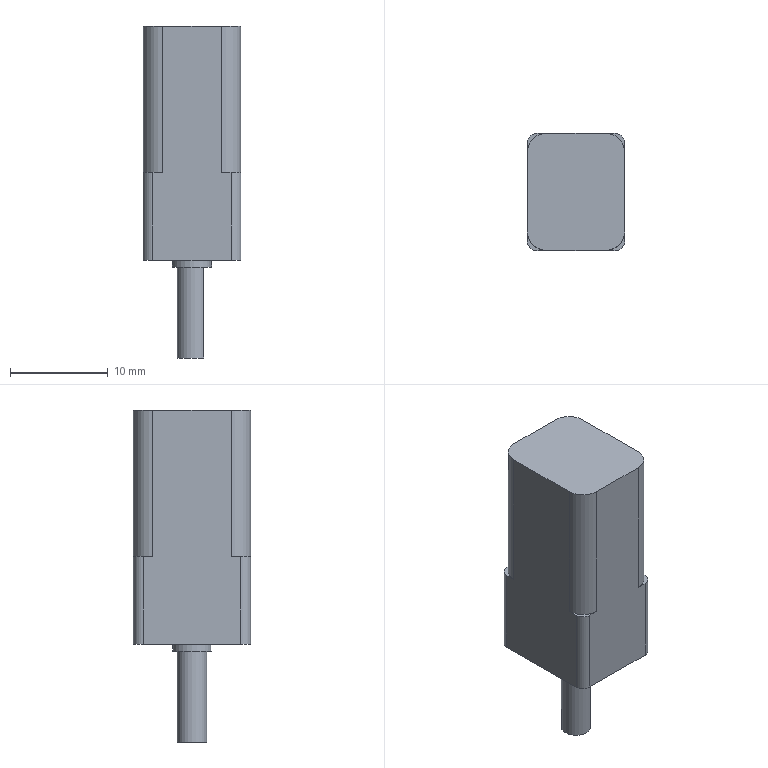Part | NX | features DATUM_CSYS 4, EXTRUDE 4, SKETCH 3, BLEND 2, UNITE 2 | 2 solids | 24 faces | box 10 x 12 x 34 mm | volume 2897 mm3 | plane 14 | cylinder 10 | commonest cylinder face diameters 4 x5 2 x4 3 x1
STEP:
#1=CARTESIAN_POINT('',(1.2,-0.9,-9.));
#2=VERTEX_POINT('',#1);
#3=CARTESIAN_POINT('',(1.2,0.9,-9.));
#4=VERTEX_POINT('',#3);
#5=CARTESIAN_POINT('',(0.,0.,-9.));
#6=DIRECTION('',(0.,0.,-1.));
#7=DIRECTION('',(1.,0.,0.));
#8=AXIS2_PLACEMENT_3D('',#5,#6,#7);
#9=CIRCLE('',#8,1.5);
#10=EDGE_CURVE('',#2,#4,#9,.T.);
#11=ORIENTED_EDGE('',*,*,#10,.T.);
#12=CARTESIAN_POINT('',(1.2,0.9,-19.));
#13=VERTEX_POINT('',#12);
#14=CARTESIAN_POINT('',(1.2,0.9,-19.));
#15=DIRECTION('',(0.,0.,1.));
#16=VECTOR('',#15,1000.);
#17=LINE('',#14,#16);
#18=EDGE_CURVE('',#13,#4,#17,.T.);
#19=ORIENTED_EDGE('',*,*,#18,.F.);
#20=CARTESIAN_POINT('',(1.2,-0.9,-19.));
#21=VERTEX_POINT('',#20);
#22=CARTESIAN_POINT('',(0.,0.,-19.));
#23=DIRECTION('',(0.,0.,-1.));
#24=DIRECTION('',(1.,0.,0.));
#25=AXIS2_PLACEMENT_3D('',#22,#23,#24);
#26=CIRCLE('',#25,1.5);
#27=EDGE_CURVE('',#21,#13,#26,.T.);
#28=ORIENTED_EDGE('',*,*,#27,.F.);
#29=CARTESIAN_POINT('',(1.2,-0.9,-19.));
#30=DIRECTION('',(0.,0.,1.));
#31=VECTOR('',#30,1000.);
#32=LINE('',#29,#31);
#33=EDGE_CURVE('',#2,#21,#32,.F.);
#34=ORIENTED_EDGE('',*,*,#33,.F.);
#35=EDGE_LOOP('',(#11,#19,#28,#34));
#36=FACE_BOUND('',#35,.T.);
#37=CARTESIAN_POINT('',(0.,0.,-19.));
#38=DIRECTION('',(0.,0.,1.));
#39=DIRECTION('',(1.,0.,0.));
#40=AXIS2_PLACEMENT_3D('',#37,#38,#39);
#41=CYLINDRICAL_SURFACE('',#40,1.5);
#42=ADVANCED_FACE('',(#36),#41,.T.);
#43=CARTESIAN_POINT('',(1.2,0.9,-9.));
#44=DIRECTION('',(0.,-1.,0.));
#45=VECTOR('',#44,1000.);
#46=LINE('',#43,#45);
#47=EDGE_CURVE('',#4,#2,#46,.T.);
#48=ORIENTED_EDGE('',*,*,#47,.T.);
#49=ORIENTED_EDGE('',*,*,#33,.T.);
#50=CARTESIAN_POINT('',(1.2,0.9,-19.));
#51=DIRECTION('',(0.,-1.,0.));
#52=VECTOR('',#51,1000.);
#53=LINE('',#50,#52);
#54=EDGE_CURVE('',#13,#21,#53,.T.);
#55=ORIENTED_EDGE('',*,*,#54,.F.);
#56=ORIENTED_EDGE('',*,*,#18,.T.);
#57=EDGE_LOOP('',(#48,#49,#55,#56));
#58=FACE_BOUND('',#57,.T.);
#59=CARTESIAN_POINT('',(1.2,0.9,-19.));
#60=DIRECTION('',(-1.,0.,0.));
#61=DIRECTION('',(0.,0.,1.));
#62=AXIS2_PLACEMENT_3D('',#59,#60,#61);
#63=PLANE('',#62);
#64=ADVANCED_FACE('',(#58),#63,.F.);
#65=ORIENTED_EDGE('',*,*,#27,.T.);
#66=ORIENTED_EDGE('',*,*,#54,.T.);
#67=EDGE_LOOP('',(#65,#66));
#68=FACE_BOUND('',#67,.T.);
#69=CARTESIAN_POINT('',(0.,0.,-19.));
#70=DIRECTION('',(0.,0.,-1.));
#71=DIRECTION('',(-1.,0.,0.));
#72=AXIS2_PLACEMENT_3D('',#69,#70,#71);
#73=PLANE('',#72);
#74=ADVANCED_FACE('',(#68),#73,.T.);
#75=ORIENTED_EDGE('',*,*,#10,.F.);
#76=ORIENTED_EDGE('',*,*,#47,.F.);
#77=EDGE_LOOP('',(#75,#76));
#78=FACE_BOUND('',#77,.T.);
#79=CARTESIAN_POINT('',(0.,0.,-9.));
#80=DIRECTION('',(0.,0.,-1.));
#81=DIRECTION('',(-1.,0.,0.));
#82=AXIS2_PLACEMENT_3D('',#79,#80,#81);
#83=PLANE('',#82);
#84=ADVANCED_FACE('',(#78),#83,.F.);
#85=CLOSED_SHELL('',(#42,#64,#74,#84));
#86=MANIFOLD_SOLID_BREP('',#85);
#87=CARTESIAN_POINT('',(2.,0.,-9.7));
#88=VERTEX_POINT('',#87);
#89=CARTESIAN_POINT('',(0.,0.,-9.7));
#90=DIRECTION('',(0.,0.,-1.));
#91=DIRECTION('',(1.,0.,0.));
#92=AXIS2_PLACEMENT_3D('',#89,#90,#91);
#93=CIRCLE('',#92,2.);
#94=EDGE_CURVE('',#88,#88,#93,.T.);
#95=ORIENTED_EDGE('',*,*,#94,.F.);
#96=EDGE_LOOP('',(#95));
#97=FACE_BOUND('',#96,.T.);
#98=CARTESIAN_POINT('',(2.,0.,-9.));
#99=VERTEX_POINT('',#98);
#100=CARTESIAN_POINT('',(0.,0.,-9.));
#101=DIRECTION('',(0.,0.,-1.));
#102=DIRECTION('',(1.,0.,0.));
#103=AXIS2_PLACEMENT_3D('',#100,#101,#102);
#104=CIRCLE('',#103,2.);
#105=EDGE_CURVE('',#99,#99,#104,.F.);
#106=ORIENTED_EDGE('',*,*,#105,.F.);
#107=EDGE_LOOP('',(#106));
#108=FACE_BOUND('',#107,.T.);
#109=CARTESIAN_POINT('',(0.,0.,-9.7));
#110=DIRECTION('',(0.,0.,1.));
#111=DIRECTION('',(1.,0.,0.));
#112=AXIS2_PLACEMENT_3D('',#109,#110,#111);
#113=CYLINDRICAL_SURFACE('',#112,2.);
#114=ADVANCED_FACE('',(#97,#108),#113,.T.);
#115=ORIENTED_EDGE('',*,*,#94,.T.);
#116=EDGE_LOOP('',(#115));
#117=FACE_BOUND('',#116,.T.);
#118=CARTESIAN_POINT('',(0.,0.,-9.7));
#119=DIRECTION('',(0.,0.,-1.));
#120=DIRECTION('',(-1.,0.,0.));
#121=AXIS2_PLACEMENT_3D('',#118,#119,#120);
#122=PLANE('',#121);
#123=ADVANCED_FACE('',(#117),#122,.T.);
#124=CARTESIAN_POINT('',(-4.,-6.,0.));
#125=VERTEX_POINT('',#124);
#126=CARTESIAN_POINT('',(-3.,-6.,0.));
#127=VERTEX_POINT('',#126);
#128=CARTESIAN_POINT('',(-5.,-6.,0.));
#129=DIRECTION('',(1.,0.,0.));
#130=VECTOR('',#129,1000.);
#131=LINE('',#128,#130);
#132=EDGE_CURVE('',#125,#127,#131,.T.);
#133=ORIENTED_EDGE('',*,*,#132,.T.);
#134=CARTESIAN_POINT('',(-5.,-4.,0.));
#135=VERTEX_POINT('',#134);
#136=CARTESIAN_POINT('',(-3.,-4.,0.));
#137=DIRECTION('',(0.,0.,1.));
#138=DIRECTION('',(1.,0.,0.));
#139=AXIS2_PLACEMENT_3D('',#136,#137,#138);
#140=CIRCLE('',#139,2.);
#141=EDGE_CURVE('',#127,#135,#140,.F.);
#142=ORIENTED_EDGE('',*,*,#141,.T.);
#143=CARTESIAN_POINT('',(-5.,-5.,0.));
#144=VERTEX_POINT('',#143);
#145=CARTESIAN_POINT('',(-5.,6.,0.));
#146=DIRECTION('',(0.,-1.,0.));
#147=VECTOR('',#146,1000.);
#148=LINE('',#145,#147);
#149=EDGE_CURVE('',#135,#144,#148,.T.);
#150=ORIENTED_EDGE('',*,*,#149,.T.);
#151=CARTESIAN_POINT('',(-4.,-5.,0.));
#152=DIRECTION('',(0.,0.,1.));
#153=DIRECTION('',(1.,0.,0.));
#154=AXIS2_PLACEMENT_3D('',#151,#152,#153);
#155=CIRCLE('',#154,1.);
#156=EDGE_CURVE('',#144,#125,#155,.T.);
#157=ORIENTED_EDGE('',*,*,#156,.T.);
#158=EDGE_LOOP('',(#133,#142,#150,#157));
#159=FACE_BOUND('',#158,.T.);
#160=CARTESIAN_POINT('',(0.,0.,0.));
#161=DIRECTION('',(0.,0.,1.));
#162=DIRECTION('',(1.,0.,0.));
#163=AXIS2_PLACEMENT_3D('',#160,#161,#162);
#164=PLANE('',#163);
#165=ADVANCED_FACE('',(#159),#164,.T.);
#166=CARTESIAN_POINT('',(-5.,5.,0.));
#167=VERTEX_POINT('',#166);
#168=CARTESIAN_POINT('',(-5.,4.,0.));
#169=VERTEX_POINT('',#168);
#170=CARTESIAN_POINT('',(-5.,6.,0.));
#171=DIRECTION('',(0.,-1.,0.));
#172=VECTOR('',#171,1000.);
#173=LINE('',#170,#172);
#174=EDGE_CURVE('',#167,#169,#173,.T.);
#175=ORIENTED_EDGE('',*,*,#174,.T.);
#176=CARTESIAN_POINT('',(-3.,6.,0.));
#177=VERTEX_POINT('',#176);
#178=CARTESIAN_POINT('',(-3.,4.,0.));
#179=DIRECTION('',(0.,0.,1.));
#180=DIRECTION('',(1.,0.,0.));
#181=AXIS2_PLACEMENT_3D('',#178,#179,#180);
#182=CIRCLE('',#181,2.);
#183=EDGE_CURVE('',#169,#177,#182,.F.);
#184=ORIENTED_EDGE('',*,*,#183,.T.);
#185=CARTESIAN_POINT('',(-4.,6.,0.));
#186=VERTEX_POINT('',#185);
#187=CARTESIAN_POINT('',(5.,6.,0.));
#188=DIRECTION('',(-1.,0.,0.));
#189=VECTOR('',#188,1000.);
#190=LINE('',#187,#189);
#191=EDGE_CURVE('',#177,#186,#190,.T.);
#192=ORIENTED_EDGE('',*,*,#191,.T.);
#193=CARTESIAN_POINT('',(-4.,5.,0.));
#194=DIRECTION('',(0.,0.,1.));
#195=DIRECTION('',(1.,0.,0.));
#196=AXIS2_PLACEMENT_3D('',#193,#194,#195);
#197=CIRCLE('',#196,1.);
#198=EDGE_CURVE('',#186,#167,#197,.T.);
#199=ORIENTED_EDGE('',*,*,#198,.T.);
#200=EDGE_LOOP('',(#175,#184,#192,#199));
#201=FACE_BOUND('',#200,.T.);
#202=CARTESIAN_POINT('',(0.,0.,0.));
#203=DIRECTION('',(0.,0.,1.));
#204=DIRECTION('',(1.,0.,0.));
#205=AXIS2_PLACEMENT_3D('',#202,#203,#204);
#206=PLANE('',#205);
#207=ADVANCED_FACE('',(#201),#206,.T.);
#208=CARTESIAN_POINT('',(4.,6.,0.));
#209=VERTEX_POINT('',#208);
#210=CARTESIAN_POINT('',(3.,6.,0.));
#211=VERTEX_POINT('',#210);
#212=CARTESIAN_POINT('',(5.,6.,0.));
#213=DIRECTION('',(-1.,0.,0.));
#214=VECTOR('',#213,1000.);
#215=LINE('',#212,#214);
#216=EDGE_CURVE('',#209,#211,#215,.T.);
#217=ORIENTED_EDGE('',*,*,#216,.T.);
#218=CARTESIAN_POINT('',(5.,4.,0.));
#219=VERTEX_POINT('',#218);
#220=CARTESIAN_POINT('',(3.,4.,0.));
#221=DIRECTION('',(0.,0.,1.));
#222=DIRECTION('',(1.,0.,0.));
#223=AXIS2_PLACEMENT_3D('',#220,#221,#222);
#224=CIRCLE('',#223,2.);
#225=EDGE_CURVE('',#211,#219,#224,.F.);
#226=ORIENTED_EDGE('',*,*,#225,.T.);
#227=CARTESIAN_POINT('',(5.,5.,0.));
#228=VERTEX_POINT('',#227);
#229=CARTESIAN_POINT('',(5.,-6.,0.));
#230=DIRECTION('',(0.,1.,0.));
#231=VECTOR('',#230,1000.);
#232=LINE('',#229,#231);
#233=EDGE_CURVE('',#219,#228,#232,.T.);
#234=ORIENTED_EDGE('',*,*,#233,.T.);
#235=CARTESIAN_POINT('',(4.,5.,0.));
#236=DIRECTION('',(0.,0.,1.));
#237=DIRECTION('',(1.,0.,0.));
#238=AXIS2_PLACEMENT_3D('',#235,#236,#237);
#239=CIRCLE('',#238,1.);
#240=EDGE_CURVE('',#228,#209,#239,.T.);
#241=ORIENTED_EDGE('',*,*,#240,.T.);
#242=EDGE_LOOP('',(#217,#226,#234,#241));
#243=FACE_BOUND('',#242,.T.);
#244=CARTESIAN_POINT('',(0.,0.,0.));
#245=DIRECTION('',(0.,0.,1.));
#246=DIRECTION('',(1.,0.,0.));
#247=AXIS2_PLACEMENT_3D('',#244,#245,#246);
#248=PLANE('',#247);
#249=ADVANCED_FACE('',(#243),#248,.T.);
#250=CARTESIAN_POINT('',(-5.,5.,-9.));
#251=VERTEX_POINT('',#250);
#252=CARTESIAN_POINT('',(-5.,-5.,-9.));
#253=VERTEX_POINT('',#252);
#254=CARTESIAN_POINT('',(-5.,6.,-9.));
#255=DIRECTION('',(0.,-1.,0.));
#256=VECTOR('',#255,1000.);
#257=LINE('',#254,#256);
#258=EDGE_CURVE('',#251,#253,#257,.T.);
#259=ORIENTED_EDGE('',*,*,#258,.T.);
#260=CARTESIAN_POINT('',(-5.,-5.,-9.));
#261=DIRECTION('',(0.,0.,1.));
#262=VECTOR('',#261,1000.);
#263=LINE('',#260,#262);
#264=EDGE_CURVE('',#253,#144,#263,.T.);
#265=ORIENTED_EDGE('',*,*,#264,.T.);
#266=ORIENTED_EDGE('',*,*,#149,.F.);
#267=CARTESIAN_POINT('',(-5.,-4.,15.));
#268=VERTEX_POINT('',#267);
#269=CARTESIAN_POINT('',(-5.,-4.,15.));
#270=DIRECTION('',(0.,0.,-1.));
#271=VECTOR('',#270,1000.);
#272=LINE('',#269,#271);
#273=EDGE_CURVE('',#135,#268,#272,.F.);
#274=ORIENTED_EDGE('',*,*,#273,.T.);
#275=CARTESIAN_POINT('',(-5.,4.,15.));
#276=VERTEX_POINT('',#275);
#277=CARTESIAN_POINT('',(-5.,6.,15.));
#278=DIRECTION('',(0.,-1.,0.));
#279=VECTOR('',#278,1000.);
#280=LINE('',#277,#279);
#281=EDGE_CURVE('',#276,#268,#280,.T.);
#282=ORIENTED_EDGE('',*,*,#281,.F.);
#283=CARTESIAN_POINT('',(-5.,4.,15.));
#284=DIRECTION('',(0.,0.,-1.));
#285=VECTOR('',#284,1000.);
#286=LINE('',#283,#285);
#287=EDGE_CURVE('',#276,#169,#286,.T.);
#288=ORIENTED_EDGE('',*,*,#287,.T.);
#289=ORIENTED_EDGE('',*,*,#174,.F.);
#290=CARTESIAN_POINT('',(-5.,5.,-9.));
#291=DIRECTION('',(0.,0.,1.));
#292=VECTOR('',#291,1000.);
#293=LINE('',#290,#292);
#294=EDGE_CURVE('',#167,#251,#293,.F.);
#295=ORIENTED_EDGE('',*,*,#294,.T.);
#296=EDGE_LOOP('',(#259,#265,#266,#274,#282,#288,#289,#295));
#297=FACE_BOUND('',#296,.T.);
#298=CARTESIAN_POINT('',(-5.,6.,-9.));
#299=DIRECTION('',(-1.,0.,0.));
#300=DIRECTION('',(0.,-1.,0.));
#301=AXIS2_PLACEMENT_3D('',#298,#299,#300);
#302=PLANE('',#301);
#303=ADVANCED_FACE('',(#297),#302,.T.);
#304=CARTESIAN_POINT('',(-4.,-6.,-9.));
#305=VERTEX_POINT('',#304);
#306=CARTESIAN_POINT('',(4.,-6.,-9.));
#307=VERTEX_POINT('',#306);
#308=CARTESIAN_POINT('',(-5.,-6.,-9.));
#309=DIRECTION('',(1.,0.,0.));
#310=VECTOR('',#309,1000.);
#311=LINE('',#308,#310);
#312=EDGE_CURVE('',#305,#307,#311,.T.);
#313=ORIENTED_EDGE('',*,*,#312,.T.);
#314=CARTESIAN_POINT('',(4.,-6.,0.));
#315=VERTEX_POINT('',#314);
#316=CARTESIAN_POINT('',(4.,-6.,-9.));
#317=DIRECTION('',(0.,0.,1.));
#318=VECTOR('',#317,1000.);
#319=LINE('',#316,#318);
#320=EDGE_CURVE('',#307,#315,#319,.T.);
#321=ORIENTED_EDGE('',*,*,#320,.T.);
#322=CARTESIAN_POINT('',(3.,-6.,0.));
#323=VERTEX_POINT('',#322);
#324=CARTESIAN_POINT('',(-5.,-6.,0.));
#325=DIRECTION('',(1.,0.,0.));
#326=VECTOR('',#325,1000.);
#327=LINE('',#324,#326);
#328=EDGE_CURVE('',#323,#315,#327,.T.);
#329=ORIENTED_EDGE('',*,*,#328,.F.);
#330=CARTESIAN_POINT('',(3.,-6.,15.));
#331=VERTEX_POINT('',#330);
#332=CARTESIAN_POINT('',(3.,-6.,15.));
#333=DIRECTION('',(0.,0.,-1.));
#334=VECTOR('',#333,1000.);
#335=LINE('',#332,#334);
#336=EDGE_CURVE('',#323,#331,#335,.F.);
#337=ORIENTED_EDGE('',*,*,#336,.T.);
#338=CARTESIAN_POINT('',(-3.,-6.,15.));
#339=VERTEX_POINT('',#338);
#340=CARTESIAN_POINT('',(-5.,-6.,15.));
#341=DIRECTION('',(1.,0.,0.));
#342=VECTOR('',#341,1000.);
#343=LINE('',#340,#342);
#344=EDGE_CURVE('',#339,#331,#343,.T.);
#345=ORIENTED_EDGE('',*,*,#344,.F.);
#346=CARTESIAN_POINT('',(-3.,-6.,15.));
#347=DIRECTION('',(0.,0.,-1.));
#348=VECTOR('',#347,1000.);
#349=LINE('',#346,#348);
#350=EDGE_CURVE('',#339,#127,#349,.T.);
#351=ORIENTED_EDGE('',*,*,#350,.T.);
#352=ORIENTED_EDGE('',*,*,#132,.F.);
#353=CARTESIAN_POINT('',(-4.,-6.,-9.));
#354=DIRECTION('',(0.,0.,1.));
#355=VECTOR('',#354,1000.);
#356=LINE('',#353,#355);
#357=EDGE_CURVE('',#125,#305,#356,.F.);
#358=ORIENTED_EDGE('',*,*,#357,.T.);
#359=EDGE_LOOP('',(#313,#321,#329,#337,#345,#351,#352,#358));
#360=FACE_BOUND('',#359,.T.);
#361=CARTESIAN_POINT('',(-5.,-6.,-9.));
#362=DIRECTION('',(0.,-1.,0.));
#363=DIRECTION('',(0.,0.,-1.));
#364=AXIS2_PLACEMENT_3D('',#361,#362,#363);
#365=PLANE('',#364);
#366=ADVANCED_FACE('',(#360),#365,.T.);
#367=CARTESIAN_POINT('',(5.,-5.,0.));
#368=VERTEX_POINT('',#367);
#369=CARTESIAN_POINT('',(5.,-4.,0.));
#370=VERTEX_POINT('',#369);
#371=CARTESIAN_POINT('',(5.,-6.,0.));
#372=DIRECTION('',(0.,1.,0.));
#373=VECTOR('',#372,1000.);
#374=LINE('',#371,#373);
#375=EDGE_CURVE('',#368,#370,#374,.T.);
#376=ORIENTED_EDGE('',*,*,#375,.F.);
#377=CARTESIAN_POINT('',(5.,-5.,-9.));
#378=VERTEX_POINT('',#377);
#379=CARTESIAN_POINT('',(5.,-5.,-9.));
#380=DIRECTION('',(0.,0.,1.));
#381=VECTOR('',#380,1000.);
#382=LINE('',#379,#381);
#383=EDGE_CURVE('',#368,#378,#382,.F.);
#384=ORIENTED_EDGE('',*,*,#383,.T.);
#385=CARTESIAN_POINT('',(5.,5.,-9.));
#386=VERTEX_POINT('',#385);
#387=CARTESIAN_POINT('',(5.,-6.,-9.));
#388=DIRECTION('',(0.,1.,0.));
#389=VECTOR('',#388,1000.);
#390=LINE('',#387,#389);
#391=EDGE_CURVE('',#378,#386,#390,.T.);
#392=ORIENTED_EDGE('',*,*,#391,.T.);
#393=CARTESIAN_POINT('',(5.,5.,-9.));
#394=DIRECTION('',(0.,0.,1.));
#395=VECTOR('',#394,1000.);
#396=LINE('',#393,#395);
#397=EDGE_CURVE('',#386,#228,#396,.T.);
#398=ORIENTED_EDGE('',*,*,#397,.T.);
#399=ORIENTED_EDGE('',*,*,#233,.F.);
#400=CARTESIAN_POINT('',(5.,4.,15.));
#401=VERTEX_POINT('',#400);
#402=CARTESIAN_POINT('',(5.,4.,15.));
#403=DIRECTION('',(0.,0.,-1.));
#404=VECTOR('',#403,1000.);
#405=LINE('',#402,#404);
#406=EDGE_CURVE('',#219,#401,#405,.F.);
#407=ORIENTED_EDGE('',*,*,#406,.T.);
#408=CARTESIAN_POINT('',(5.,-4.,15.));
#409=VERTEX_POINT('',#408);
#410=CARTESIAN_POINT('',(5.,-6.,15.));
#411=DIRECTION('',(0.,1.,0.));
#412=VECTOR('',#411,1000.);
#413=LINE('',#410,#412);
#414=EDGE_CURVE('',#409,#401,#413,.T.);
#415=ORIENTED_EDGE('',*,*,#414,.F.);
#416=CARTESIAN_POINT('',(5.,-4.,15.));
#417=DIRECTION('',(0.,0.,-1.));
#418=VECTOR('',#417,1000.);
#419=LINE('',#416,#418);
#420=EDGE_CURVE('',#409,#370,#419,.T.);
#421=ORIENTED_EDGE('',*,*,#420,.T.);
#422=EDGE_LOOP('',(#376,#384,#392,#398,#399,#407,#415,#421));
#423=FACE_BOUND('',#422,.T.);
#424=CARTESIAN_POINT('',(5.,-6.,-9.));
#425=DIRECTION('',(1.,0.,0.));
#426=DIRECTION('',(0.,1.,0.));
#427=AXIS2_PLACEMENT_3D('',#424,#425,#426);
#428=PLANE('',#427);
#429=ADVANCED_FACE('',(#423),#428,.T.);
#430=CARTESIAN_POINT('',(4.,6.,-9.));
#431=VERTEX_POINT('',#430);
#432=CARTESIAN_POINT('',(-4.,6.,-9.));
#433=VERTEX_POINT('',#432);
#434=CARTESIAN_POINT('',(5.,6.,-9.));
#435=DIRECTION('',(-1.,0.,0.));
#436=VECTOR('',#435,1000.);
#437=LINE('',#434,#436);
#438=EDGE_CURVE('',#431,#433,#437,.T.);
#439=ORIENTED_EDGE('',*,*,#438,.T.);
#440=CARTESIAN_POINT('',(-4.,6.,-9.));
#441=DIRECTION('',(0.,0.,1.));
#442=VECTOR('',#441,1000.);
#443=LINE('',#440,#442);
#444=EDGE_CURVE('',#433,#186,#443,.T.);
#445=ORIENTED_EDGE('',*,*,#444,.T.);
#446=ORIENTED_EDGE('',*,*,#191,.F.);
#447=CARTESIAN_POINT('',(-3.,6.,15.));
#448=VERTEX_POINT('',#447);
#449=CARTESIAN_POINT('',(-3.,6.,15.));
#450=DIRECTION('',(0.,0.,-1.));
#451=VECTOR('',#450,1000.);
#452=LINE('',#449,#451);
#453=EDGE_CURVE('',#177,#448,#452,.F.);
#454=ORIENTED_EDGE('',*,*,#453,.T.);
#455=CARTESIAN_POINT('',(3.,6.,15.));
#456=VERTEX_POINT('',#455);
#457=CARTESIAN_POINT('',(5.,6.,15.));
#458=DIRECTION('',(-1.,0.,0.));
#459=VECTOR('',#458,1000.);
#460=LINE('',#457,#459);
#461=EDGE_CURVE('',#456,#448,#460,.T.);
#462=ORIENTED_EDGE('',*,*,#461,.F.);
#463=CARTESIAN_POINT('',(3.,6.,15.));
#464=DIRECTION('',(0.,0.,-1.));
#465=VECTOR('',#464,1000.);
#466=LINE('',#463,#465);
#467=EDGE_CURVE('',#456,#211,#466,.T.);
#468=ORIENTED_EDGE('',*,*,#467,.T.);
#469=ORIENTED_EDGE('',*,*,#216,.F.);
#470=CARTESIAN_POINT('',(4.,6.,-9.));
#471=DIRECTION('',(0.,0.,1.));
#472=VECTOR('',#471,1000.);
#473=LINE('',#470,#472);
#474=EDGE_CURVE('',#209,#431,#473,.F.);
#475=ORIENTED_EDGE('',*,*,#474,.T.);
#476=EDGE_LOOP('',(#439,#445,#446,#454,#462,#468,#469,#475));
#477=FACE_BOUND('',#476,.T.);
#478=CARTESIAN_POINT('',(5.,6.,-9.));
#479=DIRECTION('',(0.,1.,0.));
#480=DIRECTION('',(0.,0.,1.));
#481=AXIS2_PLACEMENT_3D('',#478,#479,#480);
#482=PLANE('',#481);
#483=ADVANCED_FACE('',(#477),#482,.T.);
#484=ORIENTED_EDGE('',*,*,#105,.T.);
#485=EDGE_LOOP('',(#484));
#486=FACE_BOUND('',#485,.T.);
#487=ORIENTED_EDGE('',*,*,#391,.F.);
#488=CARTESIAN_POINT('',(4.,-5.,-9.));
#489=DIRECTION('',(0.,0.,1.));
#490=DIRECTION('',(1.,0.,0.));
#491=AXIS2_PLACEMENT_3D('',#488,#489,#490);
#492=CIRCLE('',#491,1.);
#493=EDGE_CURVE('',#378,#307,#492,.F.);
#494=ORIENTED_EDGE('',*,*,#493,.T.);
#495=ORIENTED_EDGE('',*,*,#312,.F.);
#496=CARTESIAN_POINT('',(-4.,-5.,-9.));
#497=DIRECTION('',(0.,0.,1.));
#498=DIRECTION('',(1.,0.,0.));
#499=AXIS2_PLACEMENT_3D('',#496,#497,#498);
#500=CIRCLE('',#499,1.);
#501=EDGE_CURVE('',#305,#253,#500,.F.);
#502=ORIENTED_EDGE('',*,*,#501,.T.);
#503=ORIENTED_EDGE('',*,*,#258,.F.);
#504=CARTESIAN_POINT('',(-4.,5.,-9.));
#505=DIRECTION('',(0.,0.,1.));
#506=DIRECTION('',(1.,0.,0.));
#507=AXIS2_PLACEMENT_3D('',#504,#505,#506);
#508=CIRCLE('',#507,1.);
#509=EDGE_CURVE('',#251,#433,#508,.F.);
#510=ORIENTED_EDGE('',*,*,#509,.T.);
#511=ORIENTED_EDGE('',*,*,#438,.F.);
#512=CARTESIAN_POINT('',(4.,5.,-9.));
#513=DIRECTION('',(0.,0.,1.));
#514=DIRECTION('',(1.,0.,0.));
#515=AXIS2_PLACEMENT_3D('',#512,#513,#514);
#516=CIRCLE('',#515,1.);
#517=EDGE_CURVE('',#431,#386,#516,.F.);
#518=ORIENTED_EDGE('',*,*,#517,.T.);
#519=EDGE_LOOP('',(#487,#494,#495,#502,#503,#510,#511,#518));
#520=FACE_BOUND('',#519,.T.);
#521=CARTESIAN_POINT('',(0.,0.,-9.));
#522=DIRECTION('',(0.,0.,1.));
#523=DIRECTION('',(1.,0.,0.));
#524=AXIS2_PLACEMENT_3D('',#521,#522,#523);
#525=PLANE('',#524);
#526=ADVANCED_FACE('',(#486,#520),#525,.F.);
#527=ORIENTED_EDGE('',*,*,#375,.T.);
#528=CARTESIAN_POINT('',(3.,-4.,0.));
#529=DIRECTION('',(0.,0.,1.));
#530=DIRECTION('',(1.,0.,0.));
#531=AXIS2_PLACEMENT_3D('',#528,#529,#530);
#532=CIRCLE('',#531,2.);
#533=EDGE_CURVE('',#370,#323,#532,.F.);
#534=ORIENTED_EDGE('',*,*,#533,.T.);
#535=ORIENTED_EDGE('',*,*,#328,.T.);
#536=CARTESIAN_POINT('',(4.,-5.,0.));
#537=DIRECTION('',(0.,0.,1.));
#538=DIRECTION('',(1.,0.,0.));
#539=AXIS2_PLACEMENT_3D('',#536,#537,#538);
#540=CIRCLE('',#539,1.);
#541=EDGE_CURVE('',#315,#368,#540,.T.);
#542=ORIENTED_EDGE('',*,*,#541,.T.);
#543=EDGE_LOOP('',(#527,#534,#535,#542));
#544=FACE_BOUND('',#543,.T.);
#545=CARTESIAN_POINT('',(0.,0.,0.));
#546=DIRECTION('',(0.,0.,1.));
#547=DIRECTION('',(1.,0.,0.));
#548=AXIS2_PLACEMENT_3D('',#545,#546,#547);
#549=PLANE('',#548);
#550=ADVANCED_FACE('',(#544),#549,.T.);
#551=ORIENTED_EDGE('',*,*,#493,.F.);
#552=ORIENTED_EDGE('',*,*,#383,.F.);
#553=ORIENTED_EDGE('',*,*,#541,.F.);
#554=ORIENTED_EDGE('',*,*,#320,.F.);
#555=EDGE_LOOP('',(#551,#552,#553,#554));
#556=FACE_BOUND('',#555,.T.);
#557=CARTESIAN_POINT('',(4.,-5.,-9.));
#558=DIRECTION('',(0.,0.,1.));
#559=DIRECTION('',(1.,0.,0.));
#560=AXIS2_PLACEMENT_3D('',#557,#558,#559);
#561=CYLINDRICAL_SURFACE('',#560,1.);
#562=ADVANCED_FACE('',(#556),#561,.T.);
#563=ORIENTED_EDGE('',*,*,#501,.F.);
#564=ORIENTED_EDGE('',*,*,#357,.F.);
#565=ORIENTED_EDGE('',*,*,#156,.F.);
#566=ORIENTED_EDGE('',*,*,#264,.F.);
#567=EDGE_LOOP('',(#563,#564,#565,#566));
#568=FACE_BOUND('',#567,.T.);
#569=CARTESIAN_POINT('',(-4.,-5.,-9.));
#570=DIRECTION('',(0.,0.,1.));
#571=DIRECTION('',(1.,0.,0.));
#572=AXIS2_PLACEMENT_3D('',#569,#570,#571);
#573=CYLINDRICAL_SURFACE('',#572,1.);
#574=ADVANCED_FACE('',(#568),#573,.T.);
#575=ORIENTED_EDGE('',*,*,#509,.F.);
#576=ORIENTED_EDGE('',*,*,#294,.F.);
#577=ORIENTED_EDGE('',*,*,#198,.F.);
#578=ORIENTED_EDGE('',*,*,#444,.F.);
#579=EDGE_LOOP('',(#575,#576,#577,#578));
#580=FACE_BOUND('',#579,.T.);
#581=CARTESIAN_POINT('',(-4.,5.,-9.));
#582=DIRECTION('',(0.,0.,1.));
#583=DIRECTION('',(1.,0.,0.));
#584=AXIS2_PLACEMENT_3D('',#581,#582,#583);
#585=CYLINDRICAL_SURFACE('',#584,1.);
#586=ADVANCED_FACE('',(#580),#585,.T.);
#587=ORIENTED_EDGE('',*,*,#517,.F.);
#588=ORIENTED_EDGE('',*,*,#474,.F.);
#589=ORIENTED_EDGE('',*,*,#240,.F.);
#590=ORIENTED_EDGE('',*,*,#397,.F.);
#591=EDGE_LOOP('',(#587,#588,#589,#590));
#592=FACE_BOUND('',#591,.T.);
#593=CARTESIAN_POINT('',(4.,5.,-9.));
#594=DIRECTION('',(0.,0.,1.));
#595=DIRECTION('',(1.,0.,0.));
#596=AXIS2_PLACEMENT_3D('',#593,#594,#595);
#597=CYLINDRICAL_SURFACE('',#596,1.);
#598=ADVANCED_FACE('',(#592),#597,.T.);
#599=ORIENTED_EDGE('',*,*,#281,.T.);
#600=CARTESIAN_POINT('',(-3.,-4.,15.));
#601=DIRECTION('',(0.,0.,1.));
#602=DIRECTION('',(1.,0.,0.));
#603=AXIS2_PLACEMENT_3D('',#600,#601,#602);
#604=CIRCLE('',#603,2.);
#605=EDGE_CURVE('',#268,#339,#604,.T.);
#606=ORIENTED_EDGE('',*,*,#605,.T.);
#607=ORIENTED_EDGE('',*,*,#344,.T.);
#608=CARTESIAN_POINT('',(3.,-4.,15.));
#609=DIRECTION('',(0.,0.,1.));
#610=DIRECTION('',(1.,0.,0.));
#611=AXIS2_PLACEMENT_3D('',#608,#609,#610);
#612=CIRCLE('',#611,2.);
#613=EDGE_CURVE('',#331,#409,#612,.T.);
#614=ORIENTED_EDGE('',*,*,#613,.T.);
#615=ORIENTED_EDGE('',*,*,#414,.T.);
#616=CARTESIAN_POINT('',(3.,4.,15.));
#617=DIRECTION('',(0.,0.,1.));
#618=DIRECTION('',(1.,0.,0.));
#619=AXIS2_PLACEMENT_3D('',#616,#617,#618);
#620=CIRCLE('',#619,2.);
#621=EDGE_CURVE('',#401,#456,#620,.T.);
#622=ORIENTED_EDGE('',*,*,#621,.T.);
#623=ORIENTED_EDGE('',*,*,#461,.T.);
#624=CARTESIAN_POINT('',(-3.,4.,15.));
#625=DIRECTION('',(0.,0.,1.));
#626=DIRECTION('',(1.,0.,0.));
#627=AXIS2_PLACEMENT_3D('',#624,#625,#626);
#628=CIRCLE('',#627,2.);
#629=EDGE_CURVE('',#448,#276,#628,.T.);
#630=ORIENTED_EDGE('',*,*,#629,.T.);
#631=EDGE_LOOP('',(#599,#606,#607,#614,#615,#622,#623,#630));
#632=FACE_BOUND('',#631,.T.);
#633=CARTESIAN_POINT('',(0.,0.,15.));
#634=DIRECTION('',(0.,0.,1.));
#635=DIRECTION('',(1.,0.,0.));
#636=AXIS2_PLACEMENT_3D('',#633,#634,#635);
#637=PLANE('',#636);
#638=ADVANCED_FACE('',(#632),#637,.T.);
#639=ORIENTED_EDGE('',*,*,#605,.F.);
#640=ORIENTED_EDGE('',*,*,#273,.F.);
#641=ORIENTED_EDGE('',*,*,#141,.F.);
#642=ORIENTED_EDGE('',*,*,#350,.F.);
#643=EDGE_LOOP('',(#639,#640,#641,#642));
#644=FACE_BOUND('',#643,.T.);
#645=CARTESIAN_POINT('',(-3.,-4.,15.));
#646=DIRECTION('',(0.,0.,-1.));
#647=DIRECTION('',(-1.,0.,0.));
#648=AXIS2_PLACEMENT_3D('',#645,#646,#647);
#649=CYLINDRICAL_SURFACE('',#648,2.);
#650=ADVANCED_FACE('',(#644),#649,.T.);
#651=ORIENTED_EDGE('',*,*,#613,.F.);
#652=ORIENTED_EDGE('',*,*,#336,.F.);
#653=ORIENTED_EDGE('',*,*,#533,.F.);
#654=ORIENTED_EDGE('',*,*,#420,.F.);
#655=EDGE_LOOP('',(#651,#652,#653,#654));
#656=FACE_BOUND('',#655,.T.);
#657=CARTESIAN_POINT('',(3.,-4.,15.));
#658=DIRECTION('',(0.,0.,-1.));
#659=DIRECTION('',(-1.,0.,0.));
#660=AXIS2_PLACEMENT_3D('',#657,#658,#659);
#661=CYLINDRICAL_SURFACE('',#660,2.);
#662=ADVANCED_FACE('',(#656),#661,.T.);
#663=ORIENTED_EDGE('',*,*,#621,.F.);
#664=ORIENTED_EDGE('',*,*,#406,.F.);
#665=ORIENTED_EDGE('',*,*,#225,.F.);
#666=ORIENTED_EDGE('',*,*,#467,.F.);
#667=EDGE_LOOP('',(#663,#664,#665,#666));
#668=FACE_BOUND('',#667,.T.);
#669=CARTESIAN_POINT('',(3.,4.,15.));
#670=DIRECTION('',(0.,0.,-1.));
#671=DIRECTION('',(-1.,0.,0.));
#672=AXIS2_PLACEMENT_3D('',#669,#670,#671);
#673=CYLINDRICAL_SURFACE('',#672,2.);
#674=ADVANCED_FACE('',(#668),#673,.T.);
#675=ORIENTED_EDGE('',*,*,#629,.F.);
#676=ORIENTED_EDGE('',*,*,#453,.F.);
#677=ORIENTED_EDGE('',*,*,#183,.F.);
#678=ORIENTED_EDGE('',*,*,#287,.F.);
#679=EDGE_LOOP('',(#675,#676,#677,#678));
#680=FACE_BOUND('',#679,.T.);
#681=CARTESIAN_POINT('',(-3.,4.,15.));
#682=DIRECTION('',(0.,0.,-1.));
#683=DIRECTION('',(-1.,0.,0.));
#684=AXIS2_PLACEMENT_3D('',#681,#682,#683);
#685=CYLINDRICAL_SURFACE('',#684,2.);
#686=ADVANCED_FACE('',(#680),#685,.T.);
#687=CLOSED_SHELL('',(#114,#123,#165,#207,#249,#303,#366,#429,#483,#526,#550,#562,#574,#586,#598,#638,#650,#662,#674,#686));
#688=MANIFOLD_SOLID_BREP('',#687);
#689=(LENGTH_UNIT()NAMED_UNIT(*)SI_UNIT(.MILLI.,.METRE.));
#690=UNCERTAINTY_MEASURE_WITH_UNIT(LENGTH_MEASURE(0.00001),#689,'','');
#691=(NAMED_UNIT(*)PLANE_ANGLE_UNIT()SI_UNIT($,.RADIAN.));
#692=(NAMED_UNIT(*)SI_UNIT($,.STERADIAN.)SOLID_ANGLE_UNIT());
#693=(GEOMETRIC_REPRESENTATION_CONTEXT(3)GLOBAL_UNCERTAINTY_ASSIGNED_CONTEXT((#690))GLOBAL_UNIT_ASSIGNED_CONTEXT((#689,#691,#692))REPRESENTATION_CONTEXT('',''));
#694=ADVANCED_BREP_SHAPE_REPRESENTATION('',(#86,#688),#693);